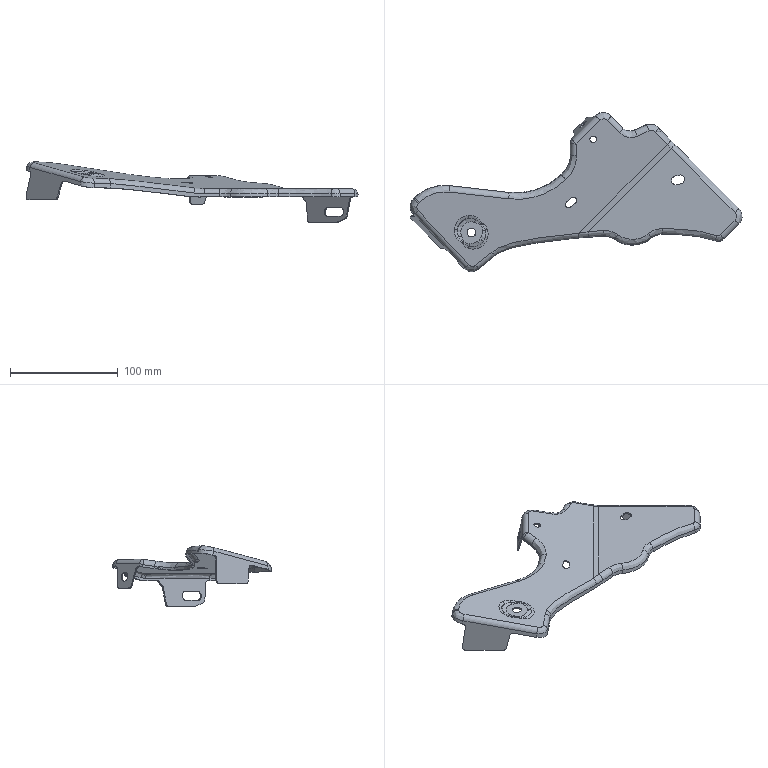Part | STEP file | 9805823380.1BPIECE_SOLIDE_FINALE_id1126_x_t | 1 solid | 245 faces | box 308.018 x 147.7 x 55.936 mm | volume 34010 mm3 | spline 175 | cylinder 48 | plane 16 | other 4 | sphere 2 | commonest cylinder face diameters 7.5 x10 10 x10 20 x6 8.2 x5 17.5 x5 6.2 x4